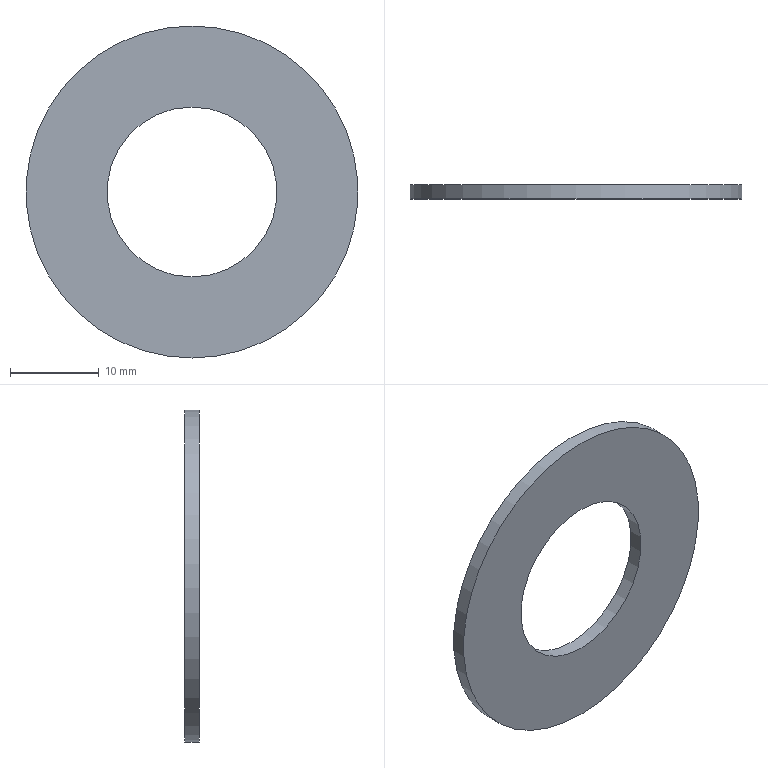Part | NX | features MG0330 trunion parts 24(trunion group) 2 | 1 solid | 4 faces | box 37.465 x 1.588 x 37.465 mm | volume 1292 mm3 | cylinder 2 | plane 2 | commonest cylinder face diameters 19.177 x1 37.465 x1
STEP:
#1=CARTESIAN_POINT('',(0.,14.935,-9.588));
#2=VERTEX_POINT('',#1);
#3=CARTESIAN_POINT('',(0.,14.935,0.));
#4=DIRECTION('',(0.,-1.,0.));
#5=DIRECTION('',(0.,0.,-1.));
#6=AXIS2_PLACEMENT_3D('',#3,#4,#5);
#7=CIRCLE('',#6,9.588);
#8=EDGE_CURVE('',#2,#2,#7,.T.);
#9=ORIENTED_EDGE('',*,*,#8,.T.);
#10=EDGE_LOOP('',(#9));
#11=FACE_BOUND('',#10,.T.);
#12=CARTESIAN_POINT('',(0.,16.523,-9.588));
#13=VERTEX_POINT('',#12);
#14=CARTESIAN_POINT('',(0.,16.523,0.));
#15=DIRECTION('',(0.,-1.,0.));
#16=DIRECTION('',(0.,0.,-1.));
#17=AXIS2_PLACEMENT_3D('',#14,#15,#16);
#18=CIRCLE('',#17,9.588);
#19=EDGE_CURVE('',#13,#13,#18,.T.);
#20=ORIENTED_EDGE('',*,*,#19,.F.);
#21=EDGE_LOOP('',(#20));
#22=FACE_BOUND('',#21,.T.);
#23=CARTESIAN_POINT('',(0.,0.,0.));
#24=DIRECTION('',(0.,-1.,0.));
#25=DIRECTION('',(0.,0.,-1.));
#26=AXIS2_PLACEMENT_3D('',#23,#24,#25);
#27=CYLINDRICAL_SURFACE('',#26,9.588);
#28=ADVANCED_FACE('',(#11,#22),#27,.F.);
#29=CARTESIAN_POINT('',(0.,14.935,-18.733));
#30=VERTEX_POINT('',#29);
#31=CARTESIAN_POINT('',(0.,14.935,0.));
#32=DIRECTION('',(0.,-1.,0.));
#33=DIRECTION('',(0.,0.,-1.));
#34=AXIS2_PLACEMENT_3D('',#31,#32,#33);
#35=CIRCLE('',#34,18.733);
#36=EDGE_CURVE('',#30,#30,#35,.T.);
#37=ORIENTED_EDGE('',*,*,#36,.T.);
#38=EDGE_LOOP('',(#37));
#39=FACE_BOUND('',#38,.T.);
#40=ORIENTED_EDGE('',*,*,#8,.F.);
#41=EDGE_LOOP('',(#40));
#42=FACE_BOUND('',#41,.T.);
#43=CARTESIAN_POINT('',(9.588,14.935,0.));
#44=DIRECTION('',(0.,-1.,0.));
#45=DIRECTION('',(0.,0.,-1.));
#46=AXIS2_PLACEMENT_3D('',#43,#44,#45);
#47=PLANE('',#46);
#48=ADVANCED_FACE('',(#39,#42),#47,.T.);
#49=CARTESIAN_POINT('',(0.,16.523,-18.733));
#50=VERTEX_POINT('',#49);
#51=CARTESIAN_POINT('',(0.,16.523,0.));
#52=DIRECTION('',(0.,-1.,0.));
#53=DIRECTION('',(0.,0.,-1.));
#54=AXIS2_PLACEMENT_3D('',#51,#52,#53);
#55=CIRCLE('',#54,18.733);
#56=EDGE_CURVE('',#50,#50,#55,.T.);
#57=ORIENTED_EDGE('',*,*,#56,.T.);
#58=EDGE_LOOP('',(#57));
#59=FACE_BOUND('',#58,.T.);
#60=ORIENTED_EDGE('',*,*,#36,.F.);
#61=EDGE_LOOP('',(#60));
#62=FACE_BOUND('',#61,.T.);
#63=CARTESIAN_POINT('',(0.,0.,0.));
#64=DIRECTION('',(0.,-1.,0.));
#65=DIRECTION('',(0.,0.,-1.));
#66=AXIS2_PLACEMENT_3D('',#63,#64,#65);
#67=CYLINDRICAL_SURFACE('',#66,18.733);
#68=ADVANCED_FACE('',(#59,#62),#67,.T.);
#69=ORIENTED_EDGE('',*,*,#19,.T.);
#70=EDGE_LOOP('',(#69));
#71=FACE_BOUND('',#70,.T.);
#72=ORIENTED_EDGE('',*,*,#56,.F.);
#73=EDGE_LOOP('',(#72));
#74=FACE_BOUND('',#73,.T.);
#75=CARTESIAN_POINT('',(9.588,16.523,0.));
#76=DIRECTION('',(0.,1.,0.));
#77=DIRECTION('',(0.,0.,1.));
#78=AXIS2_PLACEMENT_3D('',#75,#76,#77);
#79=PLANE('',#78);
#80=ADVANCED_FACE('',(#71,#74),#79,.T.);
#81=CLOSED_SHELL('',(#28,#48,#68,#80));
#82=MANIFOLD_SOLID_BREP('',#81);
#83=(LENGTH_UNIT()NAMED_UNIT(*)SI_UNIT(.MILLI.,.METRE.));
#84=UNCERTAINTY_MEASURE_WITH_UNIT(LENGTH_MEASURE(0.00001),#83,'','');
#85=(NAMED_UNIT(*)PLANE_ANGLE_UNIT()SI_UNIT($,.RADIAN.));
#86=(NAMED_UNIT(*)SI_UNIT($,.STERADIAN.)SOLID_ANGLE_UNIT());
#87=(GEOMETRIC_REPRESENTATION_CONTEXT(3)GLOBAL_UNCERTAINTY_ASSIGNED_CONTEXT((#84))GLOBAL_UNIT_ASSIGNED_CONTEXT((#83,#85,#86))REPRESENTATION_CONTEXT('',''));
#88=ADVANCED_BREP_SHAPE_REPRESENTATION('',(#82),#87);